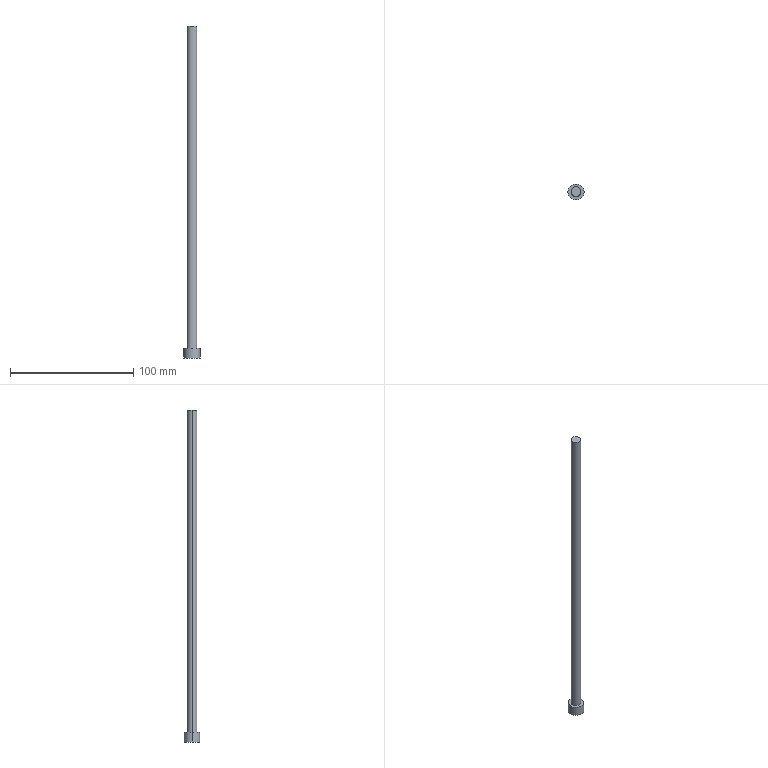Part | Creo | 1 solid | 7 faces | box 13 x 13 x 269.601 mm | volume 14211 mm3 | cylinder 4 | plane 3 | commonest cylinder face diameters 8 x2 13 x2
STEP:
#1=CARTESIAN_POINT('',(0.,0.,0.));
#2=DIRECTION('',(0.,0.,1.));
#3=DIRECTION('',(1.,0.,0.));
#4=AXIS2_PLACEMENT_3D('',#1,#2,#3);
#5=CARTESIAN_POINT('',(33.,-11.,-217.5));
#6=VERTEX_POINT('',#5);
#7=CARTESIAN_POINT('',(41.,-11.,-217.5));
#8=VERTEX_POINT('',#7);
#9=CARTESIAN_POINT('',(37.,-11.,-217.5));
#10=DIRECTION('',(0.,0.,-1.));
#11=DIRECTION('',(-1.,0.,0.));
#12=AXIS2_PLACEMENT_3D('',#9,#10,#11);
#13=CIRCLE('',#12,4.);
#14=EDGE_CURVE('',#6,#8,#13,.T.);
#15=ORIENTED_EDGE('',*,*,#14,.T.);
#16=CARTESIAN_POINT('',(41.,-11.,44.101));
#17=VERTEX_POINT('',#16);
#18=CARTESIAN_POINT('',(41.,-11.,44.101));
#19=DIRECTION('',(0.,0.,-1.));
#20=VECTOR('',#19,261.601);
#21=LINE('',#18,#20);
#22=EDGE_CURVE('',#17,#8,#21,.T.);
#23=ORIENTED_EDGE('',*,*,#22,.F.);
#24=CARTESIAN_POINT('',(33.,-11.,44.101));
#25=VERTEX_POINT('',#24);
#26=CARTESIAN_POINT('',(37.,-11.,44.101));
#27=DIRECTION('',(0.,0.,1.));
#28=DIRECTION('',(1.,0.,0.));
#29=AXIS2_PLACEMENT_3D('',#26,#27,#28);
#30=CIRCLE('',#29,4.);
#31=EDGE_CURVE('',#17,#25,#30,.T.);
#32=ORIENTED_EDGE('',*,*,#31,.T.);
#33=CARTESIAN_POINT('',(33.,-11.,44.101));
#34=DIRECTION('',(0.,0.,-1.));
#35=VECTOR('',#34,261.601);
#36=LINE('',#33,#35);
#37=EDGE_CURVE('',#25,#6,#36,.T.);
#38=ORIENTED_EDGE('',*,*,#37,.T.);
#39=EDGE_LOOP('',(#15,#23,#32,#38));
#40=FACE_OUTER_BOUND('',#39,.F.);
#41=CARTESIAN_POINT('',(37.,-11.,125.91));
#42=DIRECTION('',(0.,0.,-1.));
#43=DIRECTION('',(-1.,0.,0.));
#44=AXIS2_PLACEMENT_3D('',#41,#42,#43);
#45=CYLINDRICAL_SURFACE('',#44,4.);
#46=ADVANCED_FACE('',(#40),#45,.T.);
#47=CARTESIAN_POINT('',(30.5,-11.,-217.5));
#48=VERTEX_POINT('',#47);
#49=CARTESIAN_POINT('',(43.5,-11.,-217.5));
#50=VERTEX_POINT('',#49);
#51=CARTESIAN_POINT('',(37.,-11.,-217.5));
#52=DIRECTION('',(0.,0.,1.));
#53=DIRECTION('',(-1.,0.,0.));
#54=AXIS2_PLACEMENT_3D('',#51,#52,#53);
#55=CIRCLE('',#54,6.5);
#56=EDGE_CURVE('',#48,#50,#55,.T.);
#57=ORIENTED_EDGE('',*,*,#56,.F.);
#58=CARTESIAN_POINT('',(37.,-11.,-217.5));
#59=DIRECTION('',(0.,0.,1.));
#60=DIRECTION('',(1.,0.,0.));
#61=AXIS2_PLACEMENT_3D('',#58,#59,#60);
#62=CIRCLE('',#61,6.5);
#63=EDGE_CURVE('',#50,#48,#62,.T.);
#64=ORIENTED_EDGE('',*,*,#63,.F.);
#65=EDGE_LOOP('',(#57,#64));
#66=FACE_OUTER_BOUND('',#65,.F.);
#67=ORIENTED_EDGE('',*,*,#14,.F.);
#68=CARTESIAN_POINT('',(37.,-11.,-217.5));
#69=DIRECTION('',(0.,0.,-1.));
#70=DIRECTION('',(1.,0.,0.));
#71=AXIS2_PLACEMENT_3D('',#68,#69,#70);
#72=CIRCLE('',#71,4.);
#73=EDGE_CURVE('',#8,#6,#72,.T.);
#74=ORIENTED_EDGE('',*,*,#73,.F.);
#75=EDGE_LOOP('',(#67,#74));
#76=FACE_BOUND('',#75,.F.);
#77=CARTESIAN_POINT('',(0.,-2.5,-217.5));
#78=DIRECTION('',(0.,0.,-1.));
#79=DIRECTION('',(-1.,0.,0.));
#80=AXIS2_PLACEMENT_3D('',#77,#78,#79);
#81=PLANE('',#80);
#82=ADVANCED_FACE('',(#66,#76),#81,.F.);
#83=CARTESIAN_POINT('',(43.5,-11.,-225.5));
#84=VERTEX_POINT('',#83);
#85=CARTESIAN_POINT('',(30.5,-11.,-225.5));
#86=VERTEX_POINT('',#85);
#87=CARTESIAN_POINT('',(37.,-11.,-225.5));
#88=DIRECTION('',(0.,0.,-1.));
#89=DIRECTION('',(1.,0.,0.));
#90=AXIS2_PLACEMENT_3D('',#87,#88,#89);
#91=CIRCLE('',#90,6.5);
#92=EDGE_CURVE('',#84,#86,#91,.T.);
#93=ORIENTED_EDGE('',*,*,#92,.T.);
#94=CARTESIAN_POINT('',(30.5,-11.,-225.5));
#95=DIRECTION('',(0.,0.,1.));
#96=VECTOR('',#95,8.);
#97=LINE('',#94,#96);
#98=EDGE_CURVE('',#86,#48,#97,.T.);
#99=ORIENTED_EDGE('',*,*,#98,.T.);
#100=ORIENTED_EDGE('',*,*,#56,.T.);
#101=CARTESIAN_POINT('',(43.5,-11.,-225.5));
#102=DIRECTION('',(0.,0.,1.));
#103=VECTOR('',#102,8.);
#104=LINE('',#101,#103);
#105=EDGE_CURVE('',#84,#50,#104,.T.);
#106=ORIENTED_EDGE('',*,*,#105,.F.);
#107=EDGE_LOOP('',(#93,#99,#100,#106));
#108=FACE_OUTER_BOUND('',#107,.F.);
#109=CARTESIAN_POINT('',(37.,-11.,-225.5));
#110=DIRECTION('',(0.,0.,1.));
#111=DIRECTION('',(1.,0.,0.));
#112=AXIS2_PLACEMENT_3D('',#109,#110,#111);
#113=CYLINDRICAL_SURFACE('',#112,6.5);
#114=ADVANCED_FACE('',(#108),#113,.T.);
#115=CARTESIAN_POINT('',(37.,-11.,-225.5));
#116=DIRECTION('',(0.,0.,-1.));
#117=DIRECTION('',(-1.,0.,0.));
#118=AXIS2_PLACEMENT_3D('',#115,#116,#117);
#119=CIRCLE('',#118,6.5);
#120=EDGE_CURVE('',#86,#84,#119,.T.);
#121=ORIENTED_EDGE('',*,*,#120,.F.);
#122=ORIENTED_EDGE('',*,*,#92,.F.);
#123=EDGE_LOOP('',(#121,#122));
#124=FACE_OUTER_BOUND('',#123,.F.);
#125=CARTESIAN_POINT('',(0.,-2.5,-225.5));
#126=DIRECTION('',(0.,0.,-1.));
#127=DIRECTION('',(-1.,0.,0.));
#128=AXIS2_PLACEMENT_3D('',#125,#126,#127);
#129=PLANE('',#128);
#130=ADVANCED_FACE('',(#124),#129,.T.);
#131=ORIENTED_EDGE('',*,*,#120,.T.);
#132=ORIENTED_EDGE('',*,*,#105,.T.);
#133=ORIENTED_EDGE('',*,*,#63,.T.);
#134=ORIENTED_EDGE('',*,*,#98,.F.);
#135=EDGE_LOOP('',(#131,#132,#133,#134));
#136=FACE_OUTER_BOUND('',#135,.F.);
#137=CARTESIAN_POINT('',(37.,-11.,-225.5));
#138=DIRECTION('',(0.,0.,1.));
#139=DIRECTION('',(1.,0.,0.));
#140=AXIS2_PLACEMENT_3D('',#137,#138,#139);
#141=CYLINDRICAL_SURFACE('',#140,6.5);
#142=ADVANCED_FACE('',(#136),#141,.T.);
#143=ORIENTED_EDGE('',*,*,#73,.T.);
#144=ORIENTED_EDGE('',*,*,#37,.F.);
#145=CARTESIAN_POINT('',(37.,-11.,44.101));
#146=DIRECTION('',(0.,0.,1.));
#147=DIRECTION('',(-1.,0.,0.));
#148=AXIS2_PLACEMENT_3D('',#145,#146,#147);
#149=CIRCLE('',#148,4.);
#150=EDGE_CURVE('',#25,#17,#149,.T.);
#151=ORIENTED_EDGE('',*,*,#150,.T.);
#152=ORIENTED_EDGE('',*,*,#22,.T.);
#153=EDGE_LOOP('',(#143,#144,#151,#152));
#154=FACE_OUTER_BOUND('',#153,.F.);
#155=CARTESIAN_POINT('',(37.,-11.,125.91));
#156=DIRECTION('',(0.,0.,-1.));
#157=DIRECTION('',(-1.,0.,0.));
#158=AXIS2_PLACEMENT_3D('',#155,#156,#157);
#159=CYLINDRICAL_SURFACE('',#158,4.);
#160=ADVANCED_FACE('',(#154),#159,.T.);
#161=ORIENTED_EDGE('',*,*,#31,.F.);
#162=ORIENTED_EDGE('',*,*,#150,.F.);
#163=EDGE_LOOP('',(#161,#162));
#164=FACE_OUTER_BOUND('',#163,.F.);
#165=CARTESIAN_POINT('',(31.263,-0.4181,44.101));
#166=DIRECTION('',(0.,0.,1.));
#167=DIRECTION('',(1.,0.,0.));
#168=AXIS2_PLACEMENT_3D('',#165,#166,#167);
#169=PLANE('',#168);
#170=ADVANCED_FACE('',(#164),#169,.T.);
#171=CLOSED_SHELL('',(#46,#82,#114,#130,#142,#160,#170));
#172=MANIFOLD_SOLID_BREP('',#171);
#173=(LENGTH_UNIT()NAMED_UNIT(*)SI_UNIT(.MILLI.,.METRE.));
#174=UNCERTAINTY_MEASURE_WITH_UNIT(LENGTH_MEASURE(0.02702),#173,'','');
#175=(NAMED_UNIT(*)PLANE_ANGLE_UNIT()SI_UNIT($,.RADIAN.));
#176=PLANE_ANGLE_MEASURE_WITH_UNIT(PLANE_ANGLE_MEASURE(0.01745),#175);
#177=(CONVERSION_BASED_UNIT('DEGREE',#176)NAMED_UNIT(*)PLANE_ANGLE_UNIT());
#178=(NAMED_UNIT(*)SI_UNIT($,.STERADIAN.)SOLID_ANGLE_UNIT());
#179=(GEOMETRIC_REPRESENTATION_CONTEXT(3)GLOBAL_UNCERTAINTY_ASSIGNED_CONTEXT((#174))GLOBAL_UNIT_ASSIGNED_CONTEXT((#173,#177,#178))REPRESENTATION_CONTEXT('',''));
#180=ADVANCED_BREP_SHAPE_REPRESENTATION('',(#4,#172),#179);